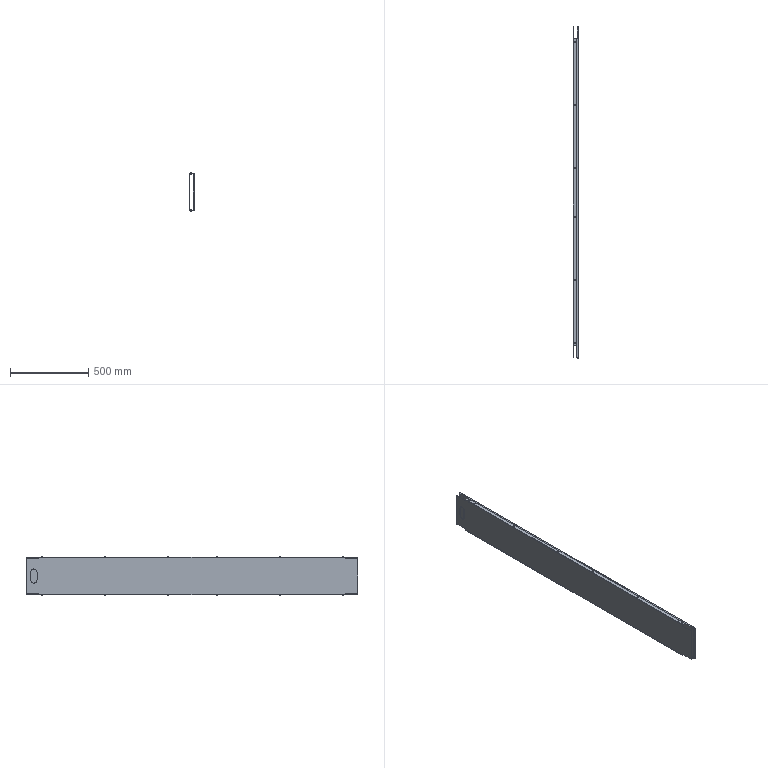Part | SolidWorks | features ReferencePattern 7, MirrorCompFeat 2 | 16 solids | 303 faces | box 36 x 2116 x 253 mm | volume 1667556 mm3 | plane 164 | cylinder 139 | commonest cylinder face diameters 6 x32 6.2 x24 8 x24 8.2 x24 12 x24 0.4 x4